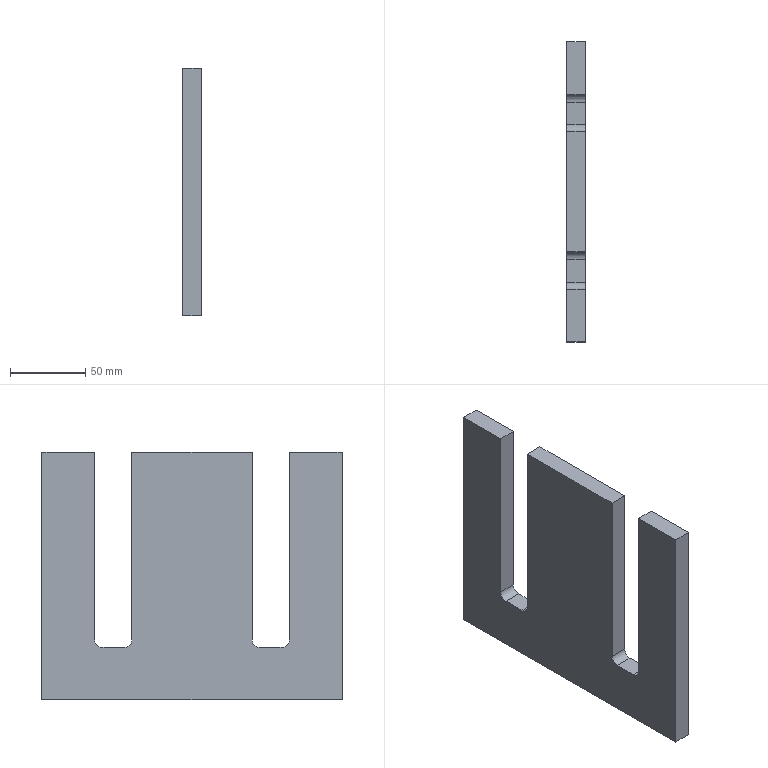Part | SolidWorks | features Extrusion 1 | 1 solid | 18 faces | box 12 x 200 x 165 mm | volume 318258 mm3 | plane 14 | cylinder 4 | commonest cylinder face diameters 10 x4
STEP:
#1=CARTESIAN_POINT('',(-140.77,-173.,-58.));
#2=VERTEX_POINT('',#1);
#3=CARTESIAN_POINT('',(-140.77,-168.,-63.));
#4=VERTEX_POINT('',#3);
#5=CARTESIAN_POINT('',(-140.77,-168.,-58.));
#6=DIRECTION('',(1.,0.,0.));
#7=DIRECTION('',(0.,0.,1.));
#8=AXIS2_PLACEMENT_3D('',#5,#6,#7);
#9=CIRCLE('',#8,5.);
#10=EDGE_CURVE('',#2,#4,#9,.T.);
#11=ORIENTED_EDGE('',*,*,#10,.T.);
#12=CARTESIAN_POINT('',(-152.77,-168.,-63.));
#13=VERTEX_POINT('',#12);
#14=CARTESIAN_POINT('',(-152.77,-168.,-63.));
#15=DIRECTION('',(1.,0.,0.));
#16=VECTOR('',#15,1000.);
#17=LINE('',#14,#16);
#18=EDGE_CURVE('',#13,#4,#17,.T.);
#19=ORIENTED_EDGE('',*,*,#18,.F.);
#20=CARTESIAN_POINT('',(-152.77,-173.,-58.));
#21=VERTEX_POINT('',#20);
#22=CARTESIAN_POINT('',(-152.77,-168.,-58.));
#23=DIRECTION('',(1.,0.,0.));
#24=DIRECTION('',(0.,0.,1.));
#25=AXIS2_PLACEMENT_3D('',#22,#23,#24);
#26=CIRCLE('',#25,5.);
#27=EDGE_CURVE('',#21,#13,#26,.T.);
#28=ORIENTED_EDGE('',*,*,#27,.F.);
#29=CARTESIAN_POINT('',(-152.77,-173.,-58.));
#30=DIRECTION('',(1.,0.,0.));
#31=VECTOR('',#30,1000.);
#32=LINE('',#29,#31);
#33=EDGE_CURVE('',#21,#2,#32,.T.);
#34=ORIENTED_EDGE('',*,*,#33,.T.);
#35=EDGE_LOOP('',(#11,#19,#28,#34));
#36=FACE_OUTER_BOUND('',#35,.T.);
#37=CARTESIAN_POINT('',(-152.77,-168.,-58.));
#38=DIRECTION('',(1.,0.,0.));
#39=DIRECTION('',(0.,0.,-1.));
#40=AXIS2_PLACEMENT_3D('',#37,#38,#39);
#41=CYLINDRICAL_SURFACE('',#40,5.);
#42=ADVANCED_FACE('',(#36),#41,.F.);
#43=CARTESIAN_POINT('',(-140.77,-153.,-63.));
#44=VERTEX_POINT('',#43);
#45=CARTESIAN_POINT('',(-140.77,-168.,-63.));
#46=DIRECTION('',(0.,1.,0.));
#47=VECTOR('',#46,1000.);
#48=LINE('',#45,#47);
#49=EDGE_CURVE('',#4,#44,#48,.T.);
#50=ORIENTED_EDGE('',*,*,#49,.T.);
#51=CARTESIAN_POINT('',(-152.77,-153.,-63.));
#52=VERTEX_POINT('',#51);
#53=CARTESIAN_POINT('',(-152.77,-153.,-63.));
#54=DIRECTION('',(1.,0.,0.));
#55=VECTOR('',#54,1000.);
#56=LINE('',#53,#55);
#57=EDGE_CURVE('',#52,#44,#56,.T.);
#58=ORIENTED_EDGE('',*,*,#57,.F.);
#59=CARTESIAN_POINT('',(-152.77,-168.,-63.));
#60=DIRECTION('',(0.,1.,0.));
#61=VECTOR('',#60,1000.);
#62=LINE('',#59,#61);
#63=EDGE_CURVE('',#13,#52,#62,.T.);
#64=ORIENTED_EDGE('',*,*,#63,.F.);
#65=ORIENTED_EDGE('',*,*,#18,.T.);
#66=EDGE_LOOP('',(#50,#58,#64,#65));
#67=FACE_OUTER_BOUND('',#66,.T.);
#68=CARTESIAN_POINT('',(-152.77,-168.,-63.));
#69=DIRECTION('',(0.,0.,-1.));
#70=DIRECTION('',(-1.,0.,0.));
#71=AXIS2_PLACEMENT_3D('',#68,#69,#70);
#72=PLANE('',#71);
#73=ADVANCED_FACE('',(#67),#72,.F.);
#74=CARTESIAN_POINT('',(-140.77,-148.,-58.));
#75=VERTEX_POINT('',#74);
#76=CARTESIAN_POINT('',(-140.77,-153.,-58.));
#77=DIRECTION('',(1.,0.,0.));
#78=DIRECTION('',(0.,0.,1.));
#79=AXIS2_PLACEMENT_3D('',#76,#77,#78);
#80=CIRCLE('',#79,5.);
#81=EDGE_CURVE('',#44,#75,#80,.T.);
#82=ORIENTED_EDGE('',*,*,#81,.T.);
#83=CARTESIAN_POINT('',(-152.77,-148.,-58.));
#84=VERTEX_POINT('',#83);
#85=CARTESIAN_POINT('',(-152.77,-148.,-58.));
#86=DIRECTION('',(1.,0.,0.));
#87=VECTOR('',#86,1000.);
#88=LINE('',#85,#87);
#89=EDGE_CURVE('',#84,#75,#88,.T.);
#90=ORIENTED_EDGE('',*,*,#89,.F.);
#91=CARTESIAN_POINT('',(-152.77,-153.,-58.));
#92=DIRECTION('',(1.,0.,0.));
#93=DIRECTION('',(0.,0.,1.));
#94=AXIS2_PLACEMENT_3D('',#91,#92,#93);
#95=CIRCLE('',#94,5.);
#96=EDGE_CURVE('',#52,#84,#95,.T.);
#97=ORIENTED_EDGE('',*,*,#96,.F.);
#98=ORIENTED_EDGE('',*,*,#57,.T.);
#99=EDGE_LOOP('',(#82,#90,#97,#98));
#100=FACE_OUTER_BOUND('',#99,.T.);
#101=CARTESIAN_POINT('',(-152.77,-153.,-58.));
#102=DIRECTION('',(1.,0.,0.));
#103=DIRECTION('',(0.,0.,-1.));
#104=AXIS2_PLACEMENT_3D('',#101,#102,#103);
#105=CYLINDRICAL_SURFACE('',#104,5.);
#106=ADVANCED_FACE('',(#100),#105,.F.);
#107=CARTESIAN_POINT('',(-140.77,-148.,67.));
#108=VERTEX_POINT('',#107);
#109=CARTESIAN_POINT('',(-140.77,-148.,-58.));
#110=DIRECTION('',(0.,0.,1.));
#111=VECTOR('',#110,1000.);
#112=LINE('',#109,#111);
#113=EDGE_CURVE('',#75,#108,#112,.T.);
#114=ORIENTED_EDGE('',*,*,#113,.T.);
#115=CARTESIAN_POINT('',(-152.77,-148.,67.));
#116=VERTEX_POINT('',#115);
#117=CARTESIAN_POINT('',(-152.77,-148.,67.));
#118=DIRECTION('',(1.,0.,0.));
#119=VECTOR('',#118,1000.);
#120=LINE('',#117,#119);
#121=EDGE_CURVE('',#116,#108,#120,.T.);
#122=ORIENTED_EDGE('',*,*,#121,.F.);
#123=CARTESIAN_POINT('',(-152.77,-148.,-58.));
#124=DIRECTION('',(0.,0.,1.));
#125=VECTOR('',#124,1000.);
#126=LINE('',#123,#125);
#127=EDGE_CURVE('',#84,#116,#126,.T.);
#128=ORIENTED_EDGE('',*,*,#127,.F.);
#129=ORIENTED_EDGE('',*,*,#89,.T.);
#130=EDGE_LOOP('',(#114,#122,#128,#129));
#131=FACE_OUTER_BOUND('',#130,.T.);
#132=CARTESIAN_POINT('',(-152.77,-148.,-58.));
#133=DIRECTION('',(0.,1.,0.));
#134=DIRECTION('',(0.,0.,1.));
#135=AXIS2_PLACEMENT_3D('',#132,#133,#134);
#136=PLANE('',#135);
#137=ADVANCED_FACE('',(#131),#136,.F.);
#138=CARTESIAN_POINT('',(-140.77,-68.,67.));
#139=VERTEX_POINT('',#138);
#140=CARTESIAN_POINT('',(-140.77,-148.,67.));
#141=DIRECTION('',(0.,1.,0.));
#142=VECTOR('',#141,1000.);
#143=LINE('',#140,#142);
#144=EDGE_CURVE('',#108,#139,#143,.T.);
#145=ORIENTED_EDGE('',*,*,#144,.T.);
#146=CARTESIAN_POINT('',(-152.77,-68.,67.));
#147=VERTEX_POINT('',#146);
#148=CARTESIAN_POINT('',(-152.77,-68.,67.));
#149=DIRECTION('',(1.,0.,0.));
#150=VECTOR('',#149,1000.);
#151=LINE('',#148,#150);
#152=EDGE_CURVE('',#147,#139,#151,.T.);
#153=ORIENTED_EDGE('',*,*,#152,.F.);
#154=CARTESIAN_POINT('',(-152.77,-148.,67.));
#155=DIRECTION('',(0.,1.,0.));
#156=VECTOR('',#155,1000.);
#157=LINE('',#154,#156);
#158=EDGE_CURVE('',#116,#147,#157,.T.);
#159=ORIENTED_EDGE('',*,*,#158,.F.);
#160=ORIENTED_EDGE('',*,*,#121,.T.);
#161=EDGE_LOOP('',(#145,#153,#159,#160));
#162=FACE_OUTER_BOUND('',#161,.T.);
#163=CARTESIAN_POINT('',(-152.77,-148.,67.));
#164=DIRECTION('',(0.,0.,-1.));
#165=DIRECTION('',(-1.,0.,0.));
#166=AXIS2_PLACEMENT_3D('',#163,#164,#165);
#167=PLANE('',#166);
#168=ADVANCED_FACE('',(#162),#167,.F.);
#169=CARTESIAN_POINT('',(-140.77,-68.,-58.));
#170=VERTEX_POINT('',#169);
#171=CARTESIAN_POINT('',(-140.77,-68.,67.));
#172=DIRECTION('',(0.,0.,-1.));
#173=VECTOR('',#172,1000.);
#174=LINE('',#171,#173);
#175=EDGE_CURVE('',#139,#170,#174,.T.);
#176=ORIENTED_EDGE('',*,*,#175,.T.);
#177=CARTESIAN_POINT('',(-152.77,-68.,-58.));
#178=VERTEX_POINT('',#177);
#179=CARTESIAN_POINT('',(-152.77,-68.,-58.));
#180=DIRECTION('',(1.,0.,0.));
#181=VECTOR('',#180,1000.);
#182=LINE('',#179,#181);
#183=EDGE_CURVE('',#178,#170,#182,.T.);
#184=ORIENTED_EDGE('',*,*,#183,.F.);
#185=CARTESIAN_POINT('',(-152.77,-68.,67.));
#186=DIRECTION('',(0.,0.,-1.));
#187=VECTOR('',#186,1000.);
#188=LINE('',#185,#187);
#189=EDGE_CURVE('',#147,#178,#188,.T.);
#190=ORIENTED_EDGE('',*,*,#189,.F.);
#191=ORIENTED_EDGE('',*,*,#152,.T.);
#192=EDGE_LOOP('',(#176,#184,#190,#191));
#193=FACE_OUTER_BOUND('',#192,.T.);
#194=CARTESIAN_POINT('',(-152.77,-68.,67.));
#195=DIRECTION('',(0.,-1.,0.));
#196=DIRECTION('',(0.,0.,-1.));
#197=AXIS2_PLACEMENT_3D('',#194,#195,#196);
#198=PLANE('',#197);
#199=ADVANCED_FACE('',(#193),#198,.F.);
#200=CARTESIAN_POINT('',(-140.77,-63.,-63.));
#201=VERTEX_POINT('',#200);
#202=CARTESIAN_POINT('',(-140.77,-63.,-58.));
#203=DIRECTION('',(1.,0.,0.));
#204=DIRECTION('',(0.,0.,1.));
#205=AXIS2_PLACEMENT_3D('',#202,#203,#204);
#206=CIRCLE('',#205,5.);
#207=EDGE_CURVE('',#170,#201,#206,.T.);
#208=ORIENTED_EDGE('',*,*,#207,.T.);
#209=CARTESIAN_POINT('',(-152.77,-63.,-63.));
#210=VERTEX_POINT('',#209);
#211=CARTESIAN_POINT('',(-152.77,-63.,-63.));
#212=DIRECTION('',(1.,0.,0.));
#213=VECTOR('',#212,1000.);
#214=LINE('',#211,#213);
#215=EDGE_CURVE('',#210,#201,#214,.T.);
#216=ORIENTED_EDGE('',*,*,#215,.F.);
#217=CARTESIAN_POINT('',(-152.77,-63.,-58.));
#218=DIRECTION('',(1.,0.,0.));
#219=DIRECTION('',(0.,0.,1.));
#220=AXIS2_PLACEMENT_3D('',#217,#218,#219);
#221=CIRCLE('',#220,5.);
#222=EDGE_CURVE('',#178,#210,#221,.T.);
#223=ORIENTED_EDGE('',*,*,#222,.F.);
#224=ORIENTED_EDGE('',*,*,#183,.T.);
#225=EDGE_LOOP('',(#208,#216,#223,#224));
#226=FACE_OUTER_BOUND('',#225,.T.);
#227=CARTESIAN_POINT('',(-152.77,-63.,-58.));
#228=DIRECTION('',(1.,0.,0.));
#229=DIRECTION('',(0.,0.,-1.));
#230=AXIS2_PLACEMENT_3D('',#227,#228,#229);
#231=CYLINDRICAL_SURFACE('',#230,5.);
#232=ADVANCED_FACE('',(#226),#231,.F.);
#233=CARTESIAN_POINT('',(-140.77,-48.,-63.));
#234=VERTEX_POINT('',#233);
#235=CARTESIAN_POINT('',(-140.77,-63.,-63.));
#236=DIRECTION('',(0.,1.,0.));
#237=VECTOR('',#236,1000.);
#238=LINE('',#235,#237);
#239=EDGE_CURVE('',#201,#234,#238,.T.);
#240=ORIENTED_EDGE('',*,*,#239,.T.);
#241=CARTESIAN_POINT('',(-152.77,-48.,-63.));
#242=VERTEX_POINT('',#241);
#243=CARTESIAN_POINT('',(-152.77,-48.,-63.));
#244=DIRECTION('',(1.,0.,0.));
#245=VECTOR('',#244,1000.);
#246=LINE('',#243,#245);
#247=EDGE_CURVE('',#242,#234,#246,.T.);
#248=ORIENTED_EDGE('',*,*,#247,.F.);
#249=CARTESIAN_POINT('',(-152.77,-63.,-63.));
#250=DIRECTION('',(0.,1.,0.));
#251=VECTOR('',#250,1000.);
#252=LINE('',#249,#251);
#253=EDGE_CURVE('',#210,#242,#252,.T.);
#254=ORIENTED_EDGE('',*,*,#253,.F.);
#255=ORIENTED_EDGE('',*,*,#215,.T.);
#256=EDGE_LOOP('',(#240,#248,#254,#255));
#257=FACE_OUTER_BOUND('',#256,.T.);
#258=CARTESIAN_POINT('',(-152.77,-63.,-63.));
#259=DIRECTION('',(0.,0.,-1.));
#260=DIRECTION('',(-1.,0.,0.));
#261=AXIS2_PLACEMENT_3D('',#258,#259,#260);
#262=PLANE('',#261);
#263=ADVANCED_FACE('',(#257),#262,.F.);
#264=CARTESIAN_POINT('',(-140.77,-43.,-58.));
#265=VERTEX_POINT('',#264);
#266=CARTESIAN_POINT('',(-140.77,-48.,-58.));
#267=DIRECTION('',(1.,0.,0.));
#268=DIRECTION('',(0.,0.,1.));
#269=AXIS2_PLACEMENT_3D('',#266,#267,#268);
#270=CIRCLE('',#269,5.);
#271=EDGE_CURVE('',#234,#265,#270,.T.);
#272=ORIENTED_EDGE('',*,*,#271,.T.);
#273=CARTESIAN_POINT('',(-152.77,-43.,-58.));
#274=VERTEX_POINT('',#273);
#275=CARTESIAN_POINT('',(-152.77,-43.,-58.));
#276=DIRECTION('',(1.,0.,0.));
#277=VECTOR('',#276,1000.);
#278=LINE('',#275,#277);
#279=EDGE_CURVE('',#274,#265,#278,.T.);
#280=ORIENTED_EDGE('',*,*,#279,.F.);
#281=CARTESIAN_POINT('',(-152.77,-48.,-58.));
#282=DIRECTION('',(1.,0.,0.));
#283=DIRECTION('',(0.,0.,1.));
#284=AXIS2_PLACEMENT_3D('',#281,#282,#283);
#285=CIRCLE('',#284,5.);
#286=EDGE_CURVE('',#242,#274,#285,.T.);
#287=ORIENTED_EDGE('',*,*,#286,.F.);
#288=ORIENTED_EDGE('',*,*,#247,.T.);
#289=EDGE_LOOP('',(#272,#280,#287,#288));
#290=FACE_OUTER_BOUND('',#289,.T.);
#291=CARTESIAN_POINT('',(-152.77,-48.,-58.));
#292=DIRECTION('',(1.,0.,0.));
#293=DIRECTION('',(0.,0.,-1.));
#294=AXIS2_PLACEMENT_3D('',#291,#292,#293);
#295=CYLINDRICAL_SURFACE('',#294,5.);
#296=ADVANCED_FACE('',(#290),#295,.F.);
#297=CARTESIAN_POINT('',(-140.77,-43.,67.));
#298=VERTEX_POINT('',#297);
#299=CARTESIAN_POINT('',(-140.77,-43.,-58.));
#300=DIRECTION('',(0.,0.,1.));
#301=VECTOR('',#300,1000.);
#302=LINE('',#299,#301);
#303=EDGE_CURVE('',#265,#298,#302,.T.);
#304=ORIENTED_EDGE('',*,*,#303,.T.);
#305=CARTESIAN_POINT('',(-152.77,-43.,67.));
#306=VERTEX_POINT('',#305);
#307=CARTESIAN_POINT('',(-152.77,-43.,67.));
#308=DIRECTION('',(1.,0.,0.));
#309=VECTOR('',#308,1000.);
#310=LINE('',#307,#309);
#311=EDGE_CURVE('',#306,#298,#310,.T.);
#312=ORIENTED_EDGE('',*,*,#311,.F.);
#313=CARTESIAN_POINT('',(-152.77,-43.,-58.));
#314=DIRECTION('',(0.,0.,1.));
#315=VECTOR('',#314,1000.);
#316=LINE('',#313,#315);
#317=EDGE_CURVE('',#274,#306,#316,.T.);
#318=ORIENTED_EDGE('',*,*,#317,.F.);
#319=ORIENTED_EDGE('',*,*,#279,.T.);
#320=EDGE_LOOP('',(#304,#312,#318,#319));
#321=FACE_OUTER_BOUND('',#320,.T.);
#322=CARTESIAN_POINT('',(-152.77,-43.,-58.));
#323=DIRECTION('',(0.,1.,0.));
#324=DIRECTION('',(0.,0.,1.));
#325=AXIS2_PLACEMENT_3D('',#322,#323,#324);
#326=PLANE('',#325);
#327=ADVANCED_FACE('',(#321),#326,.F.);
#328=CARTESIAN_POINT('',(-140.77,-8.,67.));
#329=VERTEX_POINT('',#328);
#330=CARTESIAN_POINT('',(-140.77,-43.,67.));
#331=DIRECTION('',(0.,1.,0.));
#332=VECTOR('',#331,1000.);
#333=LINE('',#330,#332);
#334=EDGE_CURVE('',#298,#329,#333,.T.);
#335=ORIENTED_EDGE('',*,*,#334,.T.);
#336=CARTESIAN_POINT('',(-152.77,-8.,67.));
#337=VERTEX_POINT('',#336);
#338=CARTESIAN_POINT('',(-152.77,-8.,67.));
#339=DIRECTION('',(1.,0.,0.));
#340=VECTOR('',#339,1000.);
#341=LINE('',#338,#340);
#342=EDGE_CURVE('',#337,#329,#341,.T.);
#343=ORIENTED_EDGE('',*,*,#342,.F.);
#344=CARTESIAN_POINT('',(-152.77,-43.,67.));
#345=DIRECTION('',(0.,1.,0.));
#346=VECTOR('',#345,1000.);
#347=LINE('',#344,#346);
#348=EDGE_CURVE('',#306,#337,#347,.T.);
#349=ORIENTED_EDGE('',*,*,#348,.F.);
#350=ORIENTED_EDGE('',*,*,#311,.T.);
#351=EDGE_LOOP('',(#335,#343,#349,#350));
#352=FACE_OUTER_BOUND('',#351,.T.);
#353=CARTESIAN_POINT('',(-152.77,-43.,67.));
#354=DIRECTION('',(0.,0.,-1.));
#355=DIRECTION('',(0.,1.,0.));
#356=AXIS2_PLACEMENT_3D('',#353,#354,#355);
#357=PLANE('',#356);
#358=ADVANCED_FACE('',(#352),#357,.F.);
#359=CARTESIAN_POINT('',(-140.77,-8.,-98.));
#360=VERTEX_POINT('',#359);
#361=CARTESIAN_POINT('',(-140.77,-8.,67.));
#362=DIRECTION('',(0.,0.,-1.));
#363=VECTOR('',#362,1000.);
#364=LINE('',#361,#363);
#365=EDGE_CURVE('',#329,#360,#364,.T.);
#366=ORIENTED_EDGE('',*,*,#365,.T.);
#367=CARTESIAN_POINT('',(-152.77,-8.,-98.));
#368=VERTEX_POINT('',#367);
#369=CARTESIAN_POINT('',(-152.77,-8.,-98.));
#370=DIRECTION('',(1.,0.,0.));
#371=VECTOR('',#370,1000.);
#372=LINE('',#369,#371);
#373=EDGE_CURVE('',#368,#360,#372,.T.);
#374=ORIENTED_EDGE('',*,*,#373,.F.);
#375=CARTESIAN_POINT('',(-152.77,-8.,67.));
#376=DIRECTION('',(0.,0.,-1.));
#377=VECTOR('',#376,1000.);
#378=LINE('',#375,#377);
#379=EDGE_CURVE('',#337,#368,#378,.T.);
#380=ORIENTED_EDGE('',*,*,#379,.F.);
#381=ORIENTED_EDGE('',*,*,#342,.T.);
#382=EDGE_LOOP('',(#366,#374,#380,#381));
#383=FACE_OUTER_BOUND('',#382,.T.);
#384=CARTESIAN_POINT('',(-152.77,-8.,67.));
#385=DIRECTION('',(0.,-1.,0.));
#386=DIRECTION('',(0.,0.,-1.));
#387=AXIS2_PLACEMENT_3D('',#384,#385,#386);
#388=PLANE('',#387);
#389=ADVANCED_FACE('',(#383),#388,.F.);
#390=CARTESIAN_POINT('',(-140.77,-208.,-98.));
#391=VERTEX_POINT('',#390);
#392=CARTESIAN_POINT('',(-140.77,-8.,-98.));
#393=DIRECTION('',(0.,-1.,0.));
#394=VECTOR('',#393,1000.);
#395=LINE('',#392,#394);
#396=EDGE_CURVE('',#360,#391,#395,.T.);
#397=ORIENTED_EDGE('',*,*,#396,.T.);
#398=CARTESIAN_POINT('',(-152.77,-208.,-98.));
#399=VERTEX_POINT('',#398);
#400=CARTESIAN_POINT('',(-152.77,-208.,-98.));
#401=DIRECTION('',(1.,0.,0.));
#402=VECTOR('',#401,1000.);
#403=LINE('',#400,#402);
#404=EDGE_CURVE('',#399,#391,#403,.T.);
#405=ORIENTED_EDGE('',*,*,#404,.F.);
#406=CARTESIAN_POINT('',(-152.77,-8.,-98.));
#407=DIRECTION('',(0.,-1.,0.));
#408=VECTOR('',#407,1000.);
#409=LINE('',#406,#408);
#410=EDGE_CURVE('',#368,#399,#409,.T.);
#411=ORIENTED_EDGE('',*,*,#410,.F.);
#412=ORIENTED_EDGE('',*,*,#373,.T.);
#413=EDGE_LOOP('',(#397,#405,#411,#412));
#414=FACE_OUTER_BOUND('',#413,.T.);
#415=CARTESIAN_POINT('',(-152.77,-8.,-98.));
#416=DIRECTION('',(0.,0.,1.));
#417=DIRECTION('',(0.,-1.,0.));
#418=AXIS2_PLACEMENT_3D('',#415,#416,#417);
#419=PLANE('',#418);
#420=ADVANCED_FACE('',(#414),#419,.F.);
#421=CARTESIAN_POINT('',(-140.77,-208.,67.));
#422=VERTEX_POINT('',#421);
#423=CARTESIAN_POINT('',(-140.77,-208.,-98.));
#424=DIRECTION('',(0.,0.,1.));
#425=VECTOR('',#424,1000.);
#426=LINE('',#423,#425);
#427=EDGE_CURVE('',#391,#422,#426,.T.);
#428=ORIENTED_EDGE('',*,*,#427,.T.);
#429=CARTESIAN_POINT('',(-152.77,-208.,67.));
#430=VERTEX_POINT('',#429);
#431=CARTESIAN_POINT('',(-152.77,-208.,67.));
#432=DIRECTION('',(1.,0.,0.));
#433=VECTOR('',#432,1000.);
#434=LINE('',#431,#433);
#435=EDGE_CURVE('',#430,#422,#434,.T.);
#436=ORIENTED_EDGE('',*,*,#435,.F.);
#437=CARTESIAN_POINT('',(-152.77,-208.,-98.));
#438=DIRECTION('',(0.,0.,1.));
#439=VECTOR('',#438,1000.);
#440=LINE('',#437,#439);
#441=EDGE_CURVE('',#399,#430,#440,.T.);
#442=ORIENTED_EDGE('',*,*,#441,.F.);
#443=ORIENTED_EDGE('',*,*,#404,.T.);
#444=EDGE_LOOP('',(#428,#436,#442,#443));
#445=FACE_OUTER_BOUND('',#444,.T.);
#446=CARTESIAN_POINT('',(-152.77,-208.,-98.));
#447=DIRECTION('',(0.,1.,0.));
#448=DIRECTION('',(0.,0.,1.));
#449=AXIS2_PLACEMENT_3D('',#446,#447,#448);
#450=PLANE('',#449);
#451=ADVANCED_FACE('',(#445),#450,.F.);
#452=CARTESIAN_POINT('',(-140.77,-173.,67.));
#453=VERTEX_POINT('',#452);
#454=CARTESIAN_POINT('',(-140.77,-208.,67.));
#455=DIRECTION('',(0.,1.,0.));
#456=VECTOR('',#455,1000.);
#457=LINE('',#454,#456);
#458=EDGE_CURVE('',#422,#453,#457,.T.);
#459=ORIENTED_EDGE('',*,*,#458,.T.);
#460=CARTESIAN_POINT('',(-152.77,-173.,67.));
#461=VERTEX_POINT('',#460);
#462=CARTESIAN_POINT('',(-152.77,-173.,67.));
#463=DIRECTION('',(1.,0.,0.));
#464=VECTOR('',#463,1000.);
#465=LINE('',#462,#464);
#466=EDGE_CURVE('',#461,#453,#465,.T.);
#467=ORIENTED_EDGE('',*,*,#466,.F.);
#468=CARTESIAN_POINT('',(-152.77,-208.,67.));
#469=DIRECTION('',(0.,1.,0.));
#470=VECTOR('',#469,1000.);
#471=LINE('',#468,#470);
#472=EDGE_CURVE('',#430,#461,#471,.T.);
#473=ORIENTED_EDGE('',*,*,#472,.F.);
#474=ORIENTED_EDGE('',*,*,#435,.T.);
#475=EDGE_LOOP('',(#459,#467,#473,#474));
#476=FACE_OUTER_BOUND('',#475,.T.);
#477=CARTESIAN_POINT('',(-152.77,-208.,67.));
#478=DIRECTION('',(0.,0.,-1.));
#479=DIRECTION('',(0.,1.,0.));
#480=AXIS2_PLACEMENT_3D('',#477,#478,#479);
#481=PLANE('',#480);
#482=ADVANCED_FACE('',(#476),#481,.F.);
#483=CARTESIAN_POINT('',(-140.77,-173.,67.));
#484=DIRECTION('',(0.,0.,-1.));
#485=VECTOR('',#484,1000.);
#486=LINE('',#483,#485);
#487=EDGE_CURVE('',#453,#2,#486,.T.);
#488=ORIENTED_EDGE('',*,*,#487,.T.);
#489=ORIENTED_EDGE('',*,*,#33,.F.);
#490=CARTESIAN_POINT('',(-152.77,-173.,67.));
#491=DIRECTION('',(0.,0.,-1.));
#492=VECTOR('',#491,1000.);
#493=LINE('',#490,#492);
#494=EDGE_CURVE('',#461,#21,#493,.T.);
#495=ORIENTED_EDGE('',*,*,#494,.F.);
#496=ORIENTED_EDGE('',*,*,#466,.T.);
#497=EDGE_LOOP('',(#488,#489,#495,#496));
#498=FACE_OUTER_BOUND('',#497,.T.);
#499=CARTESIAN_POINT('',(-152.77,-173.,67.));
#500=DIRECTION('',(0.,-1.,0.));
#501=DIRECTION('',(0.,0.,-1.));
#502=AXIS2_PLACEMENT_3D('',#499,#500,#501);
#503=PLANE('',#502);
#504=ADVANCED_FACE('',(#498),#503,.F.);
#505=ORIENTED_EDGE('',*,*,#27,.T.);
#506=ORIENTED_EDGE('',*,*,#63,.T.);
#507=ORIENTED_EDGE('',*,*,#96,.T.);
#508=ORIENTED_EDGE('',*,*,#127,.T.);
#509=ORIENTED_EDGE('',*,*,#158,.T.);
#510=ORIENTED_EDGE('',*,*,#189,.T.);
#511=ORIENTED_EDGE('',*,*,#222,.T.);
#512=ORIENTED_EDGE('',*,*,#253,.T.);
#513=ORIENTED_EDGE('',*,*,#286,.T.);
#514=ORIENTED_EDGE('',*,*,#317,.T.);
#515=ORIENTED_EDGE('',*,*,#348,.T.);
#516=ORIENTED_EDGE('',*,*,#379,.T.);
#517=ORIENTED_EDGE('',*,*,#410,.T.);
#518=ORIENTED_EDGE('',*,*,#441,.T.);
#519=ORIENTED_EDGE('',*,*,#472,.T.);
#520=ORIENTED_EDGE('',*,*,#494,.T.);
#521=EDGE_LOOP('',(#505,#506,#507,#508,#509,#510,#511,#512,#513,#514,#515,#516,#517,#518,#519,#520));
#522=FACE_OUTER_BOUND('',#521,.T.);
#523=CARTESIAN_POINT('',(-152.77,-168.,-58.));
#524=DIRECTION('',(-1.,0.,0.));
#525=DIRECTION('',(0.,0.,1.));
#526=AXIS2_PLACEMENT_3D('',#523,#524,#525);
#527=PLANE('',#526);
#528=ADVANCED_FACE('',(#522),#527,.T.);
#529=ORIENTED_EDGE('',*,*,#10,.F.);
#530=ORIENTED_EDGE('',*,*,#487,.F.);
#531=ORIENTED_EDGE('',*,*,#458,.F.);
#532=ORIENTED_EDGE('',*,*,#427,.F.);
#533=ORIENTED_EDGE('',*,*,#396,.F.);
#534=ORIENTED_EDGE('',*,*,#365,.F.);
#535=ORIENTED_EDGE('',*,*,#334,.F.);
#536=ORIENTED_EDGE('',*,*,#303,.F.);
#537=ORIENTED_EDGE('',*,*,#271,.F.);
#538=ORIENTED_EDGE('',*,*,#239,.F.);
#539=ORIENTED_EDGE('',*,*,#207,.F.);
#540=ORIENTED_EDGE('',*,*,#175,.F.);
#541=ORIENTED_EDGE('',*,*,#144,.F.);
#542=ORIENTED_EDGE('',*,*,#113,.F.);
#543=ORIENTED_EDGE('',*,*,#81,.F.);
#544=ORIENTED_EDGE('',*,*,#49,.F.);
#545=EDGE_LOOP('',(#529,#530,#531,#532,#533,#534,#535,#536,#537,#538,#539,#540,#541,#542,#543,#544));
#546=FACE_OUTER_BOUND('',#545,.T.);
#547=CARTESIAN_POINT('',(-140.77,-168.,-58.));
#548=DIRECTION('',(-1.,0.,0.));
#549=DIRECTION('',(0.,0.,1.));
#550=AXIS2_PLACEMENT_3D('',#547,#548,#549);
#551=PLANE('',#550);
#552=ADVANCED_FACE('',(#546),#551,.F.);
#553=CLOSED_SHELL('',(#42,#73,#106,#137,#168,#199,#232,#263,#296,#327,#358,#389,#420,#451,#482,#504,#528,#552));
#554=MANIFOLD_SOLID_BREP('',#553);
#555=CARTESIAN_POINT('',(0.,0.,0.));
#556=DIRECTION('',(0.,0.,1.));
#557=DIRECTION('',(1.,0.,0.));
#558=AXIS2_PLACEMENT_3D('',#555,#556,#557);
#559=(LENGTH_UNIT()NAMED_UNIT(*)SI_UNIT(.MILLI.,.METRE.));
#560=UNCERTAINTY_MEASURE_WITH_UNIT(LENGTH_MEASURE(0.00001),#559,'','');
#561=(NAMED_UNIT(*)PLANE_ANGLE_UNIT()SI_UNIT($,.RADIAN.));
#562=(NAMED_UNIT(*)SI_UNIT($,.STERADIAN.)SOLID_ANGLE_UNIT());
#563=(GEOMETRIC_REPRESENTATION_CONTEXT(3)GLOBAL_UNCERTAINTY_ASSIGNED_CONTEXT((#560))GLOBAL_UNIT_ASSIGNED_CONTEXT((#559,#561,#562))REPRESENTATION_CONTEXT('',''));
#564=ADVANCED_BREP_SHAPE_REPRESENTATION('',(#554,#558),#563);